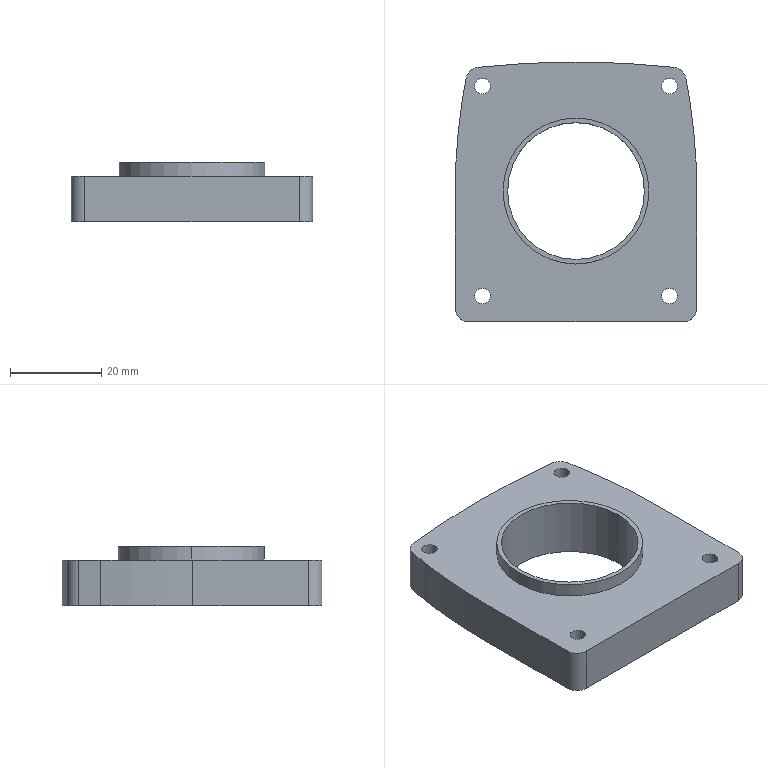Part | SolidWorks | features BaseBody 1 | 1 solid | 39 faces | box 53 x 57 x 13 mm | volume 21853 mm3 | cylinder 27 | plane 12 | commonest cylinder face diameters 6 x12 3.4 x8 30 x2 32 x2 267 x2 400 x1
STEP:
#1=CARTESIAN_POINT('',(15.,28.7,13.));
#2=VERTEX_POINT('',#1);
#3=CARTESIAN_POINT('',(-15.,28.7,13.));
#4=VERTEX_POINT('',#3);
#5=CARTESIAN_POINT('',(0.,28.7,13.));
#6=DIRECTION('',(0.,0.,-1.));
#7=DIRECTION('',(-1.,0.,0.));
#8=AXIS2_PLACEMENT_3D('',#5,#6,#7);
#9=CIRCLE('',#8,15.);
#10=EDGE_CURVE('',#2,#4,#9,.T.);
#11=ORIENTED_EDGE('',*,*,#10,.F.);
#12=CARTESIAN_POINT('',(15.,28.7,0.));
#13=VERTEX_POINT('',#12);
#14=CARTESIAN_POINT('',(15.,28.7,13.));
#15=DIRECTION('',(0.,0.,-1.));
#16=VECTOR('',#15,1000.);
#17=LINE('',#14,#16);
#18=EDGE_CURVE('',#2,#13,#17,.T.);
#19=ORIENTED_EDGE('',*,*,#18,.T.);
#20=CARTESIAN_POINT('',(-15.,28.7,0.));
#21=VERTEX_POINT('',#20);
#22=CARTESIAN_POINT('',(0.,28.7,0.));
#23=DIRECTION('',(0.,0.,-1.));
#24=DIRECTION('',(-1.,0.,0.));
#25=AXIS2_PLACEMENT_3D('',#22,#23,#24);
#26=CIRCLE('',#25,15.);
#27=EDGE_CURVE('',#13,#21,#26,.T.);
#28=ORIENTED_EDGE('',*,*,#27,.T.);
#29=CARTESIAN_POINT('',(-15.,28.7,13.));
#30=DIRECTION('',(0.,0.,-1.));
#31=VECTOR('',#30,1000.);
#32=LINE('',#29,#31);
#33=EDGE_CURVE('',#4,#21,#32,.T.);
#34=ORIENTED_EDGE('',*,*,#33,.F.);
#35=EDGE_LOOP('',(#11,#19,#28,#34));
#36=FACE_OUTER_BOUND('',#35,.T.);
#37=CARTESIAN_POINT('',(0.,28.7,13.));
#38=DIRECTION('',(0.,0.,-1.));
#39=DIRECTION('',(-1.,0.,0.));
#40=AXIS2_PLACEMENT_3D('',#37,#38,#39);
#41=CYLINDRICAL_SURFACE('',#40,15.);
#42=ADVANCED_FACE('',(#36),#41,.F.);
#43=CARTESIAN_POINT('',(-17.5,51.7,4.5));
#44=VERTEX_POINT('',#43);
#45=CARTESIAN_POINT('',(-23.5,51.7,4.5));
#46=VERTEX_POINT('',#45);
#47=CARTESIAN_POINT('',(-20.5,51.7,4.5));
#48=DIRECTION('',(0.,0.,-1.));
#49=DIRECTION('',(-1.,0.,0.));
#50=AXIS2_PLACEMENT_3D('',#47,#48,#49);
#51=CIRCLE('',#50,3.);
#52=EDGE_CURVE('',#44,#46,#51,.T.);
#53=ORIENTED_EDGE('',*,*,#52,.F.);
#54=CARTESIAN_POINT('',(-17.5,51.7,0.));
#55=VERTEX_POINT('',#54);
#56=CARTESIAN_POINT('',(-17.5,51.7,0.));
#57=DIRECTION('',(0.,0.,-1.));
#58=VECTOR('',#57,1000.);
#59=LINE('',#56,#58);
#60=EDGE_CURVE('',#44,#55,#59,.T.);
#61=ORIENTED_EDGE('',*,*,#60,.T.);
#62=CARTESIAN_POINT('',(-23.5,51.7,0.));
#63=VERTEX_POINT('',#62);
#64=CARTESIAN_POINT('',(-20.5,51.7,0.));
#65=DIRECTION('',(0.,0.,-1.));
#66=DIRECTION('',(-1.,0.,0.));
#67=AXIS2_PLACEMENT_3D('',#64,#65,#66);
#68=CIRCLE('',#67,3.);
#69=EDGE_CURVE('',#55,#63,#68,.T.);
#70=ORIENTED_EDGE('',*,*,#69,.T.);
#71=CARTESIAN_POINT('',(-23.5,51.7,0.));
#72=DIRECTION('',(0.,0.,-1.));
#73=VECTOR('',#72,1000.);
#74=LINE('',#71,#73);
#75=EDGE_CURVE('',#46,#63,#74,.T.);
#76=ORIENTED_EDGE('',*,*,#75,.F.);
#77=EDGE_LOOP('',(#53,#61,#70,#76));
#78=FACE_OUTER_BOUND('',#77,.T.);
#79=CARTESIAN_POINT('',(-20.5,51.7,0.));
#80=DIRECTION('',(0.,0.,-1.));
#81=DIRECTION('',(-1.,0.,0.));
#82=AXIS2_PLACEMENT_3D('',#79,#80,#81);
#83=CYLINDRICAL_SURFACE('',#82,3.);
#84=ADVANCED_FACE('',(#78),#83,.F.);
#85=CARTESIAN_POINT('',(-17.5,5.7,4.5));
#86=VERTEX_POINT('',#85);
#87=CARTESIAN_POINT('',(-23.5,5.7,4.5));
#88=VERTEX_POINT('',#87);
#89=CARTESIAN_POINT('',(-20.5,5.7,4.5));
#90=DIRECTION('',(0.,0.,-1.));
#91=DIRECTION('',(-1.,0.,0.));
#92=AXIS2_PLACEMENT_3D('',#89,#90,#91);
#93=CIRCLE('',#92,3.);
#94=EDGE_CURVE('',#86,#88,#93,.T.);
#95=ORIENTED_EDGE('',*,*,#94,.F.);
#96=CARTESIAN_POINT('',(-17.5,5.7,0.));
#97=VERTEX_POINT('',#96);
#98=CARTESIAN_POINT('',(-17.5,5.7,0.));
#99=DIRECTION('',(0.,0.,-1.));
#100=VECTOR('',#99,1000.);
#101=LINE('',#98,#100);
#102=EDGE_CURVE('',#86,#97,#101,.T.);
#103=ORIENTED_EDGE('',*,*,#102,.T.);
#104=CARTESIAN_POINT('',(-23.5,5.7,0.));
#105=VERTEX_POINT('',#104);
#106=CARTESIAN_POINT('',(-20.5,5.7,0.));
#107=DIRECTION('',(0.,0.,-1.));
#108=DIRECTION('',(-1.,0.,0.));
#109=AXIS2_PLACEMENT_3D('',#106,#107,#108);
#110=CIRCLE('',#109,3.);
#111=EDGE_CURVE('',#97,#105,#110,.T.);
#112=ORIENTED_EDGE('',*,*,#111,.T.);
#113=CARTESIAN_POINT('',(-23.5,5.7,0.));
#114=DIRECTION('',(0.,0.,-1.));
#115=VECTOR('',#114,1000.);
#116=LINE('',#113,#115);
#117=EDGE_CURVE('',#88,#105,#116,.T.);
#118=ORIENTED_EDGE('',*,*,#117,.F.);
#119=EDGE_LOOP('',(#95,#103,#112,#118));
#120=FACE_OUTER_BOUND('',#119,.T.);
#121=CARTESIAN_POINT('',(-20.5,5.7,0.));
#122=DIRECTION('',(0.,0.,-1.));
#123=DIRECTION('',(-1.,0.,0.));
#124=AXIS2_PLACEMENT_3D('',#121,#122,#123);
#125=CYLINDRICAL_SURFACE('',#124,3.);
#126=ADVANCED_FACE('',(#120),#125,.F.);
#127=CARTESIAN_POINT('',(23.5,5.7,4.5));
#128=VERTEX_POINT('',#127);
#129=CARTESIAN_POINT('',(17.5,5.7,4.5));
#130=VERTEX_POINT('',#129);
#131=CARTESIAN_POINT('',(20.5,5.7,4.5));
#132=DIRECTION('',(0.,0.,-1.));
#133=DIRECTION('',(-1.,0.,0.));
#134=AXIS2_PLACEMENT_3D('',#131,#132,#133);
#135=CIRCLE('',#134,3.);
#136=EDGE_CURVE('',#128,#130,#135,.T.);
#137=ORIENTED_EDGE('',*,*,#136,.F.);
#138=CARTESIAN_POINT('',(23.5,5.7,0.));
#139=VERTEX_POINT('',#138);
#140=CARTESIAN_POINT('',(23.5,5.7,0.));
#141=DIRECTION('',(0.,0.,-1.));
#142=VECTOR('',#141,1000.);
#143=LINE('',#140,#142);
#144=EDGE_CURVE('',#128,#139,#143,.T.);
#145=ORIENTED_EDGE('',*,*,#144,.T.);
#146=CARTESIAN_POINT('',(17.5,5.7,0.));
#147=VERTEX_POINT('',#146);
#148=CARTESIAN_POINT('',(20.5,5.7,0.));
#149=DIRECTION('',(0.,0.,-1.));
#150=DIRECTION('',(-1.,0.,0.));
#151=AXIS2_PLACEMENT_3D('',#148,#149,#150);
#152=CIRCLE('',#151,3.);
#153=EDGE_CURVE('',#139,#147,#152,.T.);
#154=ORIENTED_EDGE('',*,*,#153,.T.);
#155=CARTESIAN_POINT('',(17.5,5.7,0.));
#156=DIRECTION('',(0.,0.,-1.));
#157=VECTOR('',#156,1000.);
#158=LINE('',#155,#157);
#159=EDGE_CURVE('',#130,#147,#158,.T.);
#160=ORIENTED_EDGE('',*,*,#159,.F.);
#161=EDGE_LOOP('',(#137,#145,#154,#160));
#162=FACE_OUTER_BOUND('',#161,.T.);
#163=CARTESIAN_POINT('',(20.5,5.7,0.));
#164=DIRECTION('',(0.,0.,-1.));
#165=DIRECTION('',(-1.,0.,0.));
#166=AXIS2_PLACEMENT_3D('',#163,#164,#165);
#167=CYLINDRICAL_SURFACE('',#166,3.);
#168=ADVANCED_FACE('',(#162),#167,.F.);
#169=CARTESIAN_POINT('',(23.5,51.7,4.5));
#170=VERTEX_POINT('',#169);
#171=CARTESIAN_POINT('',(17.5,51.7,4.5));
#172=VERTEX_POINT('',#171);
#173=CARTESIAN_POINT('',(20.5,51.7,4.5));
#174=DIRECTION('',(0.,0.,-1.));
#175=DIRECTION('',(-1.,0.,0.));
#176=AXIS2_PLACEMENT_3D('',#173,#174,#175);
#177=CIRCLE('',#176,3.);
#178=EDGE_CURVE('',#170,#172,#177,.T.);
#179=ORIENTED_EDGE('',*,*,#178,.F.);
#180=CARTESIAN_POINT('',(23.5,51.7,0.));
#181=VERTEX_POINT('',#180);
#182=CARTESIAN_POINT('',(23.5,51.7,0.));
#183=DIRECTION('',(0.,0.,-1.));
#184=VECTOR('',#183,1000.);
#185=LINE('',#182,#184);
#186=EDGE_CURVE('',#170,#181,#185,.T.);
#187=ORIENTED_EDGE('',*,*,#186,.T.);
#188=CARTESIAN_POINT('',(17.5,51.7,0.));
#189=VERTEX_POINT('',#188);
#190=CARTESIAN_POINT('',(20.5,51.7,0.));
#191=DIRECTION('',(0.,0.,-1.));
#192=DIRECTION('',(-1.,0.,0.));
#193=AXIS2_PLACEMENT_3D('',#190,#191,#192);
#194=CIRCLE('',#193,3.);
#195=EDGE_CURVE('',#181,#189,#194,.T.);
#196=ORIENTED_EDGE('',*,*,#195,.T.);
#197=CARTESIAN_POINT('',(17.5,51.7,0.));
#198=DIRECTION('',(0.,0.,-1.));
#199=VECTOR('',#198,1000.);
#200=LINE('',#197,#199);
#201=EDGE_CURVE('',#172,#189,#200,.T.);
#202=ORIENTED_EDGE('',*,*,#201,.F.);
#203=EDGE_LOOP('',(#179,#187,#196,#202));
#204=FACE_OUTER_BOUND('',#203,.T.);
#205=CARTESIAN_POINT('',(20.5,51.7,0.));
#206=DIRECTION('',(0.,0.,-1.));
#207=DIRECTION('',(-1.,0.,0.));
#208=AXIS2_PLACEMENT_3D('',#205,#206,#207);
#209=CYLINDRICAL_SURFACE('',#208,3.);
#210=ADVANCED_FACE('',(#204),#209,.F.);
#211=CARTESIAN_POINT('',(16.,28.7,13.));
#212=VERTEX_POINT('',#211);
#213=CARTESIAN_POINT('',(-16.,28.7,13.));
#214=VERTEX_POINT('',#213);
#215=CARTESIAN_POINT('',(0.,28.7,13.));
#216=DIRECTION('',(0.,0.,1.));
#217=DIRECTION('',(-1.,0.,0.));
#218=AXIS2_PLACEMENT_3D('',#215,#216,#217);
#219=CIRCLE('',#218,16.);
#220=EDGE_CURVE('',#212,#214,#219,.T.);
#221=ORIENTED_EDGE('',*,*,#220,.F.);
#222=CARTESIAN_POINT('',(16.,28.7,10.));
#223=VERTEX_POINT('',#222);
#224=CARTESIAN_POINT('',(16.,28.7,13.));
#225=DIRECTION('',(0.,0.,-1.));
#226=VECTOR('',#225,1000.);
#227=LINE('',#224,#226);
#228=EDGE_CURVE('',#212,#223,#227,.T.);
#229=ORIENTED_EDGE('',*,*,#228,.T.);
#230=CARTESIAN_POINT('',(-16.,28.7,10.));
#231=VERTEX_POINT('',#230);
#232=CARTESIAN_POINT('',(0.,28.7,10.));
#233=DIRECTION('',(0.,0.,-1.));
#234=DIRECTION('',(-1.,0.,0.));
#235=AXIS2_PLACEMENT_3D('',#232,#233,#234);
#236=CIRCLE('',#235,16.);
#237=EDGE_CURVE('',#231,#223,#236,.T.);
#238=ORIENTED_EDGE('',*,*,#237,.F.);
#239=CARTESIAN_POINT('',(-16.,28.7,13.));
#240=DIRECTION('',(0.,0.,-1.));
#241=VECTOR('',#240,1000.);
#242=LINE('',#239,#241);
#243=EDGE_CURVE('',#214,#231,#242,.T.);
#244=ORIENTED_EDGE('',*,*,#243,.F.);
#245=EDGE_LOOP('',(#221,#229,#238,#244));
#246=FACE_OUTER_BOUND('',#245,.T.);
#247=CARTESIAN_POINT('',(0.,28.7,13.));
#248=DIRECTION('',(0.,0.,-1.));
#249=DIRECTION('',(-1.,0.,0.));
#250=AXIS2_PLACEMENT_3D('',#247,#248,#249);
#251=CYLINDRICAL_SURFACE('',#250,16.);
#252=ADVANCED_FACE('',(#246),#251,.T.);
#253=CARTESIAN_POINT('',(-18.8,51.7,10.));
#254=VERTEX_POINT('',#253);
#255=CARTESIAN_POINT('',(-22.2,51.7,10.));
#256=VERTEX_POINT('',#255);
#257=CARTESIAN_POINT('',(-20.5,51.7,10.));
#258=DIRECTION('',(0.,0.,-1.));
#259=DIRECTION('',(-1.,0.,0.));
#260=AXIS2_PLACEMENT_3D('',#257,#258,#259);
#261=CIRCLE('',#260,1.7);
#262=EDGE_CURVE('',#254,#256,#261,.T.);
#263=ORIENTED_EDGE('',*,*,#262,.F.);
#264=CARTESIAN_POINT('',(-18.8,51.7,4.5));
#265=VERTEX_POINT('',#264);
#266=CARTESIAN_POINT('',(-18.8,51.7,0.));
#267=DIRECTION('',(0.,0.,-1.));
#268=VECTOR('',#267,1000.);
#269=LINE('',#266,#268);
#270=EDGE_CURVE('',#254,#265,#269,.T.);
#271=ORIENTED_EDGE('',*,*,#270,.T.);
#272=CARTESIAN_POINT('',(-22.2,51.7,4.5));
#273=VERTEX_POINT('',#272);
#274=CARTESIAN_POINT('',(-20.5,51.7,4.5));
#275=DIRECTION('',(0.,0.,-1.));
#276=DIRECTION('',(-1.,0.,0.));
#277=AXIS2_PLACEMENT_3D('',#274,#275,#276);
#278=CIRCLE('',#277,1.7);
#279=EDGE_CURVE('',#265,#273,#278,.T.);
#280=ORIENTED_EDGE('',*,*,#279,.T.);
#281=CARTESIAN_POINT('',(-22.2,51.7,0.));
#282=DIRECTION('',(0.,0.,-1.));
#283=VECTOR('',#282,1000.);
#284=LINE('',#281,#283);
#285=EDGE_CURVE('',#256,#273,#284,.T.);
#286=ORIENTED_EDGE('',*,*,#285,.F.);
#287=EDGE_LOOP('',(#263,#271,#280,#286));
#288=FACE_OUTER_BOUND('',#287,.T.);
#289=CARTESIAN_POINT('',(-20.5,51.7,0.));
#290=DIRECTION('',(0.,0.,-1.));
#291=DIRECTION('',(-1.,0.,0.));
#292=AXIS2_PLACEMENT_3D('',#289,#290,#291);
#293=CYLINDRICAL_SURFACE('',#292,1.7);
#294=ADVANCED_FACE('',(#288),#293,.F.);
#295=CARTESIAN_POINT('',(-18.8,5.7,10.));
#296=VERTEX_POINT('',#295);
#297=CARTESIAN_POINT('',(-22.2,5.7,10.));
#298=VERTEX_POINT('',#297);
#299=CARTESIAN_POINT('',(-20.5,5.7,10.));
#300=DIRECTION('',(0.,0.,-1.));
#301=DIRECTION('',(-1.,0.,0.));
#302=AXIS2_PLACEMENT_3D('',#299,#300,#301);
#303=CIRCLE('',#302,1.7);
#304=EDGE_CURVE('',#296,#298,#303,.T.);
#305=ORIENTED_EDGE('',*,*,#304,.F.);
#306=CARTESIAN_POINT('',(-18.8,5.7,4.5));
#307=VERTEX_POINT('',#306);
#308=CARTESIAN_POINT('',(-18.8,5.7,0.));
#309=DIRECTION('',(0.,0.,-1.));
#310=VECTOR('',#309,1000.);
#311=LINE('',#308,#310);
#312=EDGE_CURVE('',#296,#307,#311,.T.);
#313=ORIENTED_EDGE('',*,*,#312,.T.);
#314=CARTESIAN_POINT('',(-22.2,5.7,4.5));
#315=VERTEX_POINT('',#314);
#316=CARTESIAN_POINT('',(-20.5,5.7,4.5));
#317=DIRECTION('',(0.,0.,-1.));
#318=DIRECTION('',(-1.,0.,0.));
#319=AXIS2_PLACEMENT_3D('',#316,#317,#318);
#320=CIRCLE('',#319,1.7);
#321=EDGE_CURVE('',#307,#315,#320,.T.);
#322=ORIENTED_EDGE('',*,*,#321,.T.);
#323=CARTESIAN_POINT('',(-22.2,5.7,0.));
#324=DIRECTION('',(0.,0.,-1.));
#325=VECTOR('',#324,1000.);
#326=LINE('',#323,#325);
#327=EDGE_CURVE('',#298,#315,#326,.T.);
#328=ORIENTED_EDGE('',*,*,#327,.F.);
#329=EDGE_LOOP('',(#305,#313,#322,#328));
#330=FACE_OUTER_BOUND('',#329,.T.);
#331=CARTESIAN_POINT('',(-20.5,5.7,0.));
#332=DIRECTION('',(0.,0.,-1.));
#333=DIRECTION('',(-1.,0.,0.));
#334=AXIS2_PLACEMENT_3D('',#331,#332,#333);
#335=CYLINDRICAL_SURFACE('',#334,1.7);
#336=ADVANCED_FACE('',(#330),#335,.F.);
#337=CARTESIAN_POINT('',(22.2,5.7,10.));
#338=VERTEX_POINT('',#337);
#339=CARTESIAN_POINT('',(18.8,5.7,10.));
#340=VERTEX_POINT('',#339);
#341=CARTESIAN_POINT('',(20.5,5.7,10.));
#342=DIRECTION('',(0.,0.,-1.));
#343=DIRECTION('',(-1.,0.,0.));
#344=AXIS2_PLACEMENT_3D('',#341,#342,#343);
#345=CIRCLE('',#344,1.7);
#346=EDGE_CURVE('',#338,#340,#345,.T.);
#347=ORIENTED_EDGE('',*,*,#346,.F.);
#348=CARTESIAN_POINT('',(22.2,5.7,4.5));
#349=VERTEX_POINT('',#348);
#350=CARTESIAN_POINT('',(22.2,5.7,0.));
#351=DIRECTION('',(0.,0.,-1.));
#352=VECTOR('',#351,1000.);
#353=LINE('',#350,#352);
#354=EDGE_CURVE('',#338,#349,#353,.T.);
#355=ORIENTED_EDGE('',*,*,#354,.T.);
#356=CARTESIAN_POINT('',(18.8,5.7,4.5));
#357=VERTEX_POINT('',#356);
#358=CARTESIAN_POINT('',(20.5,5.7,4.5));
#359=DIRECTION('',(0.,0.,-1.));
#360=DIRECTION('',(-1.,0.,0.));
#361=AXIS2_PLACEMENT_3D('',#358,#359,#360);
#362=CIRCLE('',#361,1.7);
#363=EDGE_CURVE('',#349,#357,#362,.T.);
#364=ORIENTED_EDGE('',*,*,#363,.T.);
#365=CARTESIAN_POINT('',(18.8,5.7,0.));
#366=DIRECTION('',(0.,0.,-1.));
#367=VECTOR('',#366,1000.);
#368=LINE('',#365,#367);
#369=EDGE_CURVE('',#340,#357,#368,.T.);
#370=ORIENTED_EDGE('',*,*,#369,.F.);
#371=EDGE_LOOP('',(#347,#355,#364,#370));
#372=FACE_OUTER_BOUND('',#371,.T.);
#373=CARTESIAN_POINT('',(20.5,5.7,0.));
#374=DIRECTION('',(0.,0.,-1.));
#375=DIRECTION('',(-1.,0.,0.));
#376=AXIS2_PLACEMENT_3D('',#373,#374,#375);
#377=CYLINDRICAL_SURFACE('',#376,1.7);
#378=ADVANCED_FACE('',(#372),#377,.F.);
#379=CARTESIAN_POINT('',(22.2,51.7,10.));
#380=VERTEX_POINT('',#379);
#381=CARTESIAN_POINT('',(18.8,51.7,10.));
#382=VERTEX_POINT('',#381);
#383=CARTESIAN_POINT('',(20.5,51.7,10.));
#384=DIRECTION('',(0.,0.,-1.));
#385=DIRECTION('',(-1.,0.,0.));
#386=AXIS2_PLACEMENT_3D('',#383,#384,#385);
#387=CIRCLE('',#386,1.7);
#388=EDGE_CURVE('',#380,#382,#387,.T.);
#389=ORIENTED_EDGE('',*,*,#388,.F.);
#390=CARTESIAN_POINT('',(22.2,51.7,4.5));
#391=VERTEX_POINT('',#390);
#392=CARTESIAN_POINT('',(22.2,51.7,0.));
#393=DIRECTION('',(0.,0.,-1.));
#394=VECTOR('',#393,1000.);
#395=LINE('',#392,#394);
#396=EDGE_CURVE('',#380,#391,#395,.T.);
#397=ORIENTED_EDGE('',*,*,#396,.T.);
#398=CARTESIAN_POINT('',(18.8,51.7,4.5));
#399=VERTEX_POINT('',#398);
#400=CARTESIAN_POINT('',(20.5,51.7,4.5));
#401=DIRECTION('',(0.,0.,-1.));
#402=DIRECTION('',(-1.,0.,0.));
#403=AXIS2_PLACEMENT_3D('',#400,#401,#402);
#404=CIRCLE('',#403,1.7);
#405=EDGE_CURVE('',#391,#399,#404,.T.);
#406=ORIENTED_EDGE('',*,*,#405,.T.);
#407=CARTESIAN_POINT('',(18.8,51.7,0.));
#408=DIRECTION('',(0.,0.,-1.));
#409=VECTOR('',#408,1000.);
#410=LINE('',#407,#409);
#411=EDGE_CURVE('',#382,#399,#410,.T.);
#412=ORIENTED_EDGE('',*,*,#411,.F.);
#413=EDGE_LOOP('',(#389,#397,#406,#412));
#414=FACE_OUTER_BOUND('',#413,.T.);
#415=CARTESIAN_POINT('',(20.5,51.7,0.));
#416=DIRECTION('',(0.,0.,-1.));
#417=DIRECTION('',(-1.,0.,0.));
#418=AXIS2_PLACEMENT_3D('',#415,#416,#417);
#419=CYLINDRICAL_SURFACE('',#418,1.7);
#420=ADVANCED_FACE('',(#414),#419,.F.);
#421=CARTESIAN_POINT('',(-23.5,0.,0.));
#422=VERTEX_POINT('',#421);
#423=CARTESIAN_POINT('',(23.5,0.,0.));
#424=VERTEX_POINT('',#423);
#425=CARTESIAN_POINT('',(23.5,0.,0.));
#426=DIRECTION('',(1.,0.,0.));
#427=VECTOR('',#426,1000.);
#428=LINE('',#425,#427);
#429=EDGE_CURVE('',#422,#424,#428,.T.);
#430=ORIENTED_EDGE('',*,*,#429,.F.);
#431=CARTESIAN_POINT('',(-26.5,3.,0.));
#432=VERTEX_POINT('',#431);
#433=CARTESIAN_POINT('',(-23.5,3.,0.));
#434=DIRECTION('',(0.,0.,1.));
#435=DIRECTION('',(-1.,0.,0.));
#436=AXIS2_PLACEMENT_3D('',#433,#434,#435);
#437=CIRCLE('',#436,3.);
#438=EDGE_CURVE('',#432,#422,#437,.T.);
#439=ORIENTED_EDGE('',*,*,#438,.F.);
#440=CARTESIAN_POINT('',(-26.5,28.3,0.));
#441=VERTEX_POINT('',#440);
#442=CARTESIAN_POINT('',(-26.5,3.,0.));
#443=DIRECTION('',(0.,-1.,0.));
#444=VECTOR('',#443,1000.);
#445=LINE('',#442,#444);
#446=EDGE_CURVE('',#441,#432,#445,.T.);
#447=ORIENTED_EDGE('',*,*,#446,.F.);
#448=CARTESIAN_POINT('',(-24.963,48.5,0.));
#449=VERTEX_POINT('',#448);
#450=CARTESIAN_POINT('',(107.,28.3,0.));
#451=DIRECTION('',(0.,0.,1.));
#452=DIRECTION('',(-1.,0.,0.));
#453=AXIS2_PLACEMENT_3D('',#450,#451,#452);
#454=CIRCLE('',#453,133.5);
#455=EDGE_CURVE('',#449,#441,#454,.T.);
#456=ORIENTED_EDGE('',*,*,#455,.F.);
#457=CARTESIAN_POINT('',(-24.102,53.383,0.));
#458=VERTEX_POINT('',#457);
#459=CARTESIAN_POINT('',(-24.102,53.383,0.));
#460=DIRECTION('',(-0.1736,-0.9848,0.));
#461=VECTOR('',#460,1000.);
#462=LINE('',#459,#461);
#463=EDGE_CURVE('',#458,#449,#462,.T.);
#464=ORIENTED_EDGE('',*,*,#463,.F.);
#465=CARTESIAN_POINT('',(-21.47,55.844,0.));
#466=VERTEX_POINT('',#465);
#467=CARTESIAN_POINT('',(-21.148,52.862,0.));
#468=DIRECTION('',(0.,0.,1.));
#469=DIRECTION('',(-1.,0.,0.));
#470=AXIS2_PLACEMENT_3D('',#467,#468,#469);
#471=CIRCLE('',#470,3.);
#472=EDGE_CURVE('',#466,#458,#471,.T.);
#473=ORIENTED_EDGE('',*,*,#472,.F.);
#474=CARTESIAN_POINT('',(21.47,55.844,0.));
#475=VERTEX_POINT('',#474);
#476=CARTESIAN_POINT('',(0.,-143.,0.));
#477=DIRECTION('',(0.,0.,1.));
#478=DIRECTION('',(-1.,0.,0.));
#479=AXIS2_PLACEMENT_3D('',#476,#477,#478);
#480=CIRCLE('',#479,200.);
#481=EDGE_CURVE('',#475,#466,#480,.T.);
#482=ORIENTED_EDGE('',*,*,#481,.F.);
#483=CARTESIAN_POINT('',(24.102,53.383,0.));
#484=VERTEX_POINT('',#483);
#485=CARTESIAN_POINT('',(21.148,52.862,0.));
#486=DIRECTION('',(0.,0.,1.));
#487=DIRECTION('',(-1.,0.,0.));
#488=AXIS2_PLACEMENT_3D('',#485,#486,#487);
#489=CIRCLE('',#488,3.);
#490=EDGE_CURVE('',#484,#475,#489,.T.);
#491=ORIENTED_EDGE('',*,*,#490,.F.);
#492=CARTESIAN_POINT('',(24.963,48.5,0.));
#493=VERTEX_POINT('',#492);
#494=CARTESIAN_POINT('',(24.963,48.5,0.));
#495=DIRECTION('',(-0.1736,0.9848,0.));
#496=VECTOR('',#495,1000.);
#497=LINE('',#494,#496);
#498=EDGE_CURVE('',#493,#484,#497,.T.);
#499=ORIENTED_EDGE('',*,*,#498,.F.);
#500=CARTESIAN_POINT('',(26.5,28.3,0.));
#501=VERTEX_POINT('',#500);
#502=CARTESIAN_POINT('',(-107.,28.3,0.));
#503=DIRECTION('',(0.,0.,1.));
#504=DIRECTION('',(-1.,0.,0.));
#505=AXIS2_PLACEMENT_3D('',#502,#503,#504);
#506=CIRCLE('',#505,133.5);
#507=EDGE_CURVE('',#501,#493,#506,.T.);
#508=ORIENTED_EDGE('',*,*,#507,.F.);
#509=CARTESIAN_POINT('',(26.5,3.,0.));
#510=VERTEX_POINT('',#509);
#511=CARTESIAN_POINT('',(26.5,3.,0.));
#512=DIRECTION('',(0.,1.,0.));
#513=VECTOR('',#512,1000.);
#514=LINE('',#511,#513);
#515=EDGE_CURVE('',#510,#501,#514,.T.);
#516=ORIENTED_EDGE('',*,*,#515,.F.);
#517=CARTESIAN_POINT('',(23.5,3.,0.));
#518=DIRECTION('',(0.,0.,1.));
#519=DIRECTION('',(-1.,0.,0.));
#520=AXIS2_PLACEMENT_3D('',#517,#518,#519);
#521=CIRCLE('',#520,3.);
#522=EDGE_CURVE('',#424,#510,#521,.T.);
#523=ORIENTED_EDGE('',*,*,#522,.F.);
#524=EDGE_LOOP('',(#430,#439,#447,#456,#464,#473,#482,#491,#499,#508,#516,#523));
#525=FACE_OUTER_BOUND('',#524,.T.);
#526=CARTESIAN_POINT('',(0.,28.7,0.));
#527=DIRECTION('',(0.,0.,-1.));
#528=DIRECTION('',(-1.,0.,0.));
#529=AXIS2_PLACEMENT_3D('',#526,#527,#528);
#530=CIRCLE('',#529,15.);
#531=EDGE_CURVE('',#21,#13,#530,.T.);
#532=ORIENTED_EDGE('',*,*,#531,.F.);
#533=ORIENTED_EDGE('',*,*,#27,.F.);
#534=EDGE_LOOP('',(#532,#533));
#535=FACE_BOUND('',#534,.T.);
#536=CARTESIAN_POINT('',(-20.5,51.7,0.));
#537=DIRECTION('',(0.,0.,-1.));
#538=DIRECTION('',(-1.,0.,0.));
#539=AXIS2_PLACEMENT_3D('',#536,#537,#538);
#540=CIRCLE('',#539,3.);
#541=EDGE_CURVE('',#63,#55,#540,.T.);
#542=ORIENTED_EDGE('',*,*,#541,.F.);
#543=ORIENTED_EDGE('',*,*,#69,.F.);
#544=EDGE_LOOP('',(#542,#543));
#545=FACE_BOUND('',#544,.T.);
#546=CARTESIAN_POINT('',(-20.5,5.7,0.));
#547=DIRECTION('',(0.,0.,-1.));
#548=DIRECTION('',(-1.,0.,0.));
#549=AXIS2_PLACEMENT_3D('',#546,#547,#548);
#550=CIRCLE('',#549,3.);
#551=EDGE_CURVE('',#105,#97,#550,.T.);
#552=ORIENTED_EDGE('',*,*,#551,.F.);
#553=ORIENTED_EDGE('',*,*,#111,.F.);
#554=EDGE_LOOP('',(#552,#553));
#555=FACE_BOUND('',#554,.T.);
#556=CARTESIAN_POINT('',(20.5,5.7,0.));
#557=DIRECTION('',(0.,0.,-1.));
#558=DIRECTION('',(-1.,0.,0.));
#559=AXIS2_PLACEMENT_3D('',#556,#557,#558);
#560=CIRCLE('',#559,3.);
#561=EDGE_CURVE('',#147,#139,#560,.T.);
#562=ORIENTED_EDGE('',*,*,#561,.F.);
#563=ORIENTED_EDGE('',*,*,#153,.F.);
#564=EDGE_LOOP('',(#562,#563));
#565=FACE_BOUND('',#564,.T.);
#566=CARTESIAN_POINT('',(20.5,51.7,0.));
#567=DIRECTION('',(0.,0.,-1.));
#568=DIRECTION('',(-1.,0.,0.));
#569=AXIS2_PLACEMENT_3D('',#566,#567,#568);
#570=CIRCLE('',#569,3.);
#571=EDGE_CURVE('',#189,#181,#570,.T.);
#572=ORIENTED_EDGE('',*,*,#571,.F.);
#573=ORIENTED_EDGE('',*,*,#195,.F.);
#574=EDGE_LOOP('',(#572,#573));
#575=FACE_BOUND('',#574,.T.);
#576=CARTESIAN_POINT('',(23.5,3.,0.));
#577=DIRECTION('',(0.,0.,1.));
#578=DIRECTION('',(1.,0.,0.));
#579=AXIS2_PLACEMENT_3D('',#576,#577,#578);
#580=PLANE('',#579);
#581=ADVANCED_FACE('',(#525,#535,#545,#555,#565,#575),#580,.F.);
#582=CARTESIAN_POINT('',(26.5,3.,10.));
#583=VERTEX_POINT('',#582);
#584=CARTESIAN_POINT('',(23.5,0.,10.));
#585=VERTEX_POINT('',#584);
#586=CARTESIAN_POINT('',(23.5,3.,10.));
#587=DIRECTION('',(0.,0.,-1.));
#588=DIRECTION('',(-1.,0.,0.));
#589=AXIS2_PLACEMENT_3D('',#586,#587,#588);
#590=CIRCLE('',#589,3.);
#591=EDGE_CURVE('',#583,#585,#590,.T.);
#592=ORIENTED_EDGE('',*,*,#591,.T.);
#593=CARTESIAN_POINT('',(23.5,0.,10.));
#594=DIRECTION('',(0.,0.,-1.));
#595=VECTOR('',#594,1000.);
#596=LINE('',#593,#595);
#597=EDGE_CURVE('',#585,#424,#596,.T.);
#598=ORIENTED_EDGE('',*,*,#597,.T.);
#599=ORIENTED_EDGE('',*,*,#522,.T.);
#600=CARTESIAN_POINT('',(26.5,3.,10.));
#601=DIRECTION('',(0.,0.,1.));
#602=VECTOR('',#601,1000.);
#603=LINE('',#600,#602);
#604=EDGE_CURVE('',#510,#583,#603,.T.);
#605=ORIENTED_EDGE('',*,*,#604,.T.);
#606=EDGE_LOOP('',(#592,#598,#599,#605));
#607=FACE_OUTER_BOUND('',#606,.T.);
#608=CARTESIAN_POINT('',(23.5,3.,10.));
#609=DIRECTION('',(0.,0.,-1.));
#610=DIRECTION('',(-1.,0.,0.));
#611=AXIS2_PLACEMENT_3D('',#608,#609,#610);
#612=CYLINDRICAL_SURFACE('',#611,3.);
#613=ADVANCED_FACE('',(#607),#612,.T.);
#614=ORIENTED_EDGE('',*,*,#597,.F.);
#615=CARTESIAN_POINT('',(-23.5,0.,10.));
#616=VERTEX_POINT('',#615);
#617=CARTESIAN_POINT('',(23.5,0.,10.));
#618=DIRECTION('',(1.,0.,0.));
#619=VECTOR('',#618,1000.);
#620=LINE('',#617,#619);
#621=EDGE_CURVE('',#616,#585,#620,.T.);
#622=ORIENTED_EDGE('',*,*,#621,.F.);
#623=CARTESIAN_POINT('',(-23.5,0.,10.));
#624=DIRECTION('',(0.,0.,1.));
#625=VECTOR('',#624,1000.);
#626=LINE('',#623,#625);
#627=EDGE_CURVE('',#422,#616,#626,.T.);
#628=ORIENTED_EDGE('',*,*,#627,.F.);
#629=ORIENTED_EDGE('',*,*,#429,.T.);
#630=EDGE_LOOP('',(#614,#622,#628,#629));
#631=FACE_OUTER_BOUND('',#630,.T.);
#632=CARTESIAN_POINT('',(23.5,0.,10.));
#633=DIRECTION('',(0.,1.,0.));
#634=DIRECTION('',(0.,0.,1.));
#635=AXIS2_PLACEMENT_3D('',#632,#633,#634);
#636=PLANE('',#635);
#637=ADVANCED_FACE('',(#631),#636,.F.);
#638=CARTESIAN_POINT('',(-26.5,3.,10.));
#639=VERTEX_POINT('',#638);
#640=CARTESIAN_POINT('',(-23.5,3.,10.));
#641=DIRECTION('',(0.,0.,-1.));
#642=DIRECTION('',(-1.,0.,0.));
#643=AXIS2_PLACEMENT_3D('',#640,#641,#642);
#644=CIRCLE('',#643,3.);
#645=EDGE_CURVE('',#616,#639,#644,.T.);
#646=ORIENTED_EDGE('',*,*,#645,.T.);
#647=CARTESIAN_POINT('',(-26.5,3.,10.));
#648=DIRECTION('',(0.,0.,-1.));
#649=VECTOR('',#648,1000.);
#650=LINE('',#647,#649);
#651=EDGE_CURVE('',#639,#432,#650,.T.);
#652=ORIENTED_EDGE('',*,*,#651,.T.);
#653=ORIENTED_EDGE('',*,*,#438,.T.);
#654=ORIENTED_EDGE('',*,*,#627,.T.);
#655=EDGE_LOOP('',(#646,#652,#653,#654));
#656=FACE_OUTER_BOUND('',#655,.T.);
#657=CARTESIAN_POINT('',(-23.5,3.,10.));
#658=DIRECTION('',(0.,0.,-1.));
#659=DIRECTION('',(-1.,0.,0.));
#660=AXIS2_PLACEMENT_3D('',#657,#658,#659);
#661=CYLINDRICAL_SURFACE('',#660,3.);
#662=ADVANCED_FACE('',(#656),#661,.T.);
#663=ORIENTED_EDGE('',*,*,#651,.F.);
#664=CARTESIAN_POINT('',(-26.5,28.3,10.));
#665=VERTEX_POINT('',#664);
#666=CARTESIAN_POINT('',(-26.5,3.,10.));
#667=DIRECTION('',(0.,-1.,0.));
#668=VECTOR('',#667,1000.);
#669=LINE('',#666,#668);
#670=EDGE_CURVE('',#665,#639,#669,.T.);
#671=ORIENTED_EDGE('',*,*,#670,.F.);
#672=CARTESIAN_POINT('',(-26.5,28.3,10.));
#673=DIRECTION('',(0.,0.,1.));
#674=VECTOR('',#673,1000.);
#675=LINE('',#672,#674);
#676=EDGE_CURVE('',#441,#665,#675,.T.);
#677=ORIENTED_EDGE('',*,*,#676,.F.);
#678=ORIENTED_EDGE('',*,*,#446,.T.);
#679=EDGE_LOOP('',(#663,#671,#677,#678));
#680=FACE_OUTER_BOUND('',#679,.T.);
#681=CARTESIAN_POINT('',(-26.5,3.,10.));
#682=DIRECTION('',(1.,0.,0.));
#683=DIRECTION('',(0.,0.,-1.));
#684=AXIS2_PLACEMENT_3D('',#681,#682,#683);
#685=PLANE('',#684);
#686=ADVANCED_FACE('',(#680),#685,.F.);
#687=CARTESIAN_POINT('',(-24.963,48.5,10.));
#688=VERTEX_POINT('',#687);
#689=CARTESIAN_POINT('',(107.,28.3,10.));
#690=DIRECTION('',(0.,0.,-1.));
#691=DIRECTION('',(-1.,0.,0.));
#692=AXIS2_PLACEMENT_3D('',#689,#690,#691);
#693=CIRCLE('',#692,133.5);
#694=EDGE_CURVE('',#665,#688,#693,.T.);
#695=ORIENTED_EDGE('',*,*,#694,.T.);
#696=CARTESIAN_POINT('',(-24.963,48.5,10.));
#697=DIRECTION('',(0.,0.,-1.));
#698=VECTOR('',#697,1000.);
#699=LINE('',#696,#698);
#700=EDGE_CURVE('',#688,#449,#699,.T.);
#701=ORIENTED_EDGE('',*,*,#700,.T.);
#702=ORIENTED_EDGE('',*,*,#455,.T.);
#703=ORIENTED_EDGE('',*,*,#676,.T.);
#704=EDGE_LOOP('',(#695,#701,#702,#703));
#705=FACE_OUTER_BOUND('',#704,.T.);
#706=CARTESIAN_POINT('',(107.,28.3,10.));
#707=DIRECTION('',(0.,0.,-1.));
#708=DIRECTION('',(-1.,0.,0.));
#709=AXIS2_PLACEMENT_3D('',#706,#707,#708);
#710=CYLINDRICAL_SURFACE('',#709,133.5);
#711=ADVANCED_FACE('',(#705),#710,.T.);
#712=ORIENTED_EDGE('',*,*,#700,.F.);
#713=CARTESIAN_POINT('',(-24.102,53.383,10.));
#714=VERTEX_POINT('',#713);
#715=CARTESIAN_POINT('',(-24.963,48.5,10.));
#716=DIRECTION('',(-0.1736,-0.9848,0.));
#717=VECTOR('',#716,1000.);
#718=LINE('',#715,#717);
#719=EDGE_CURVE('',#714,#688,#718,.T.);
#720=ORIENTED_EDGE('',*,*,#719,.F.);
#721=CARTESIAN_POINT('',(-24.102,53.383,10.));
#722=DIRECTION('',(0.,0.,1.));
#723=VECTOR('',#722,1000.);
#724=LINE('',#721,#723);
#725=EDGE_CURVE('',#458,#714,#724,.T.);
#726=ORIENTED_EDGE('',*,*,#725,.F.);
#727=ORIENTED_EDGE('',*,*,#463,.T.);
#728=EDGE_LOOP('',(#712,#720,#726,#727));
#729=FACE_OUTER_BOUND('',#728,.T.);
#730=CARTESIAN_POINT('',(-24.963,48.5,10.));
#731=DIRECTION('',(0.9848,-0.1736,0.));
#732=DIRECTION('',(0.1736,0.9848,0.));
#733=AXIS2_PLACEMENT_3D('',#730,#731,#732);
#734=PLANE('',#733);
#735=ADVANCED_FACE('',(#729),#734,.F.);
#736=CARTESIAN_POINT('',(-21.47,55.844,10.));
#737=VERTEX_POINT('',#736);
#738=CARTESIAN_POINT('',(-21.148,52.862,10.));
#739=DIRECTION('',(0.,0.,-1.));
#740=DIRECTION('',(-1.,0.,0.));
#741=AXIS2_PLACEMENT_3D('',#738,#739,#740);
#742=CIRCLE('',#741,3.);
#743=EDGE_CURVE('',#714,#737,#742,.T.);
#744=ORIENTED_EDGE('',*,*,#743,.T.);
#745=CARTESIAN_POINT('',(-21.47,55.844,10.));
#746=DIRECTION('',(0.,0.,-1.));
#747=VECTOR('',#746,1000.);
#748=LINE('',#745,#747);
#749=EDGE_CURVE('',#737,#466,#748,.T.);
#750=ORIENTED_EDGE('',*,*,#749,.T.);
#751=ORIENTED_EDGE('',*,*,#472,.T.);
#752=ORIENTED_EDGE('',*,*,#725,.T.);
#753=EDGE_LOOP('',(#744,#750,#751,#752));
#754=FACE_OUTER_BOUND('',#753,.T.);
#755=CARTESIAN_POINT('',(-21.148,52.862,10.));
#756=DIRECTION('',(0.,0.,-1.));
#757=DIRECTION('',(-1.,0.,0.));
#758=AXIS2_PLACEMENT_3D('',#755,#756,#757);
#759=CYLINDRICAL_SURFACE('',#758,3.);
#760=ADVANCED_FACE('',(#754),#759,.T.);
#761=CARTESIAN_POINT('',(21.47,55.844,10.));
#762=VERTEX_POINT('',#761);
#763=CARTESIAN_POINT('',(0.,-143.,10.));
#764=DIRECTION('',(0.,0.,-1.));
#765=DIRECTION('',(-1.,0.,0.));
#766=AXIS2_PLACEMENT_3D('',#763,#764,#765);
#767=CIRCLE('',#766,200.);
#768=EDGE_CURVE('',#737,#762,#767,.T.);
#769=ORIENTED_EDGE('',*,*,#768,.T.);
#770=CARTESIAN_POINT('',(21.47,55.844,10.));
#771=DIRECTION('',(0.,0.,-1.));
#772=VECTOR('',#771,1000.);
#773=LINE('',#770,#772);
#774=EDGE_CURVE('',#762,#475,#773,.T.);
#775=ORIENTED_EDGE('',*,*,#774,.T.);
#776=ORIENTED_EDGE('',*,*,#481,.T.);
#777=ORIENTED_EDGE('',*,*,#749,.F.);
#778=EDGE_LOOP('',(#769,#775,#776,#777));
#779=FACE_OUTER_BOUND('',#778,.T.);
#780=CARTESIAN_POINT('',(0.,-143.,10.));
#781=DIRECTION('',(0.,0.,-1.));
#782=DIRECTION('',(-1.,0.,0.));
#783=AXIS2_PLACEMENT_3D('',#780,#781,#782);
#784=CYLINDRICAL_SURFACE('',#783,200.);
#785=ADVANCED_FACE('',(#779),#784,.T.);
#786=CARTESIAN_POINT('',(24.102,53.383,10.));
#787=VERTEX_POINT('',#786);
#788=CARTESIAN_POINT('',(21.148,52.862,10.));
#789=DIRECTION('',(0.,0.,-1.));
#790=DIRECTION('',(-1.,0.,0.));
#791=AXIS2_PLACEMENT_3D('',#788,#789,#790);
#792=CIRCLE('',#791,3.);
#793=EDGE_CURVE('',#762,#787,#792,.T.);
#794=ORIENTED_EDGE('',*,*,#793,.T.);
#795=CARTESIAN_POINT('',(24.102,53.383,10.));
#796=DIRECTION('',(0.,0.,-1.));
#797=VECTOR('',#796,1000.);
#798=LINE('',#795,#797);
#799=EDGE_CURVE('',#787,#484,#798,.T.);
#800=ORIENTED_EDGE('',*,*,#799,.T.);
#801=ORIENTED_EDGE('',*,*,#490,.T.);
#802=ORIENTED_EDGE('',*,*,#774,.F.);
#803=EDGE_LOOP('',(#794,#800,#801,#802));
#804=FACE_OUTER_BOUND('',#803,.T.);
#805=CARTESIAN_POINT('',(21.148,52.862,10.));
#806=DIRECTION('',(0.,0.,-1.));
#807=DIRECTION('',(-1.,0.,0.));
#808=AXIS2_PLACEMENT_3D('',#805,#806,#807);
#809=CYLINDRICAL_SURFACE('',#808,3.);
#810=ADVANCED_FACE('',(#804),#809,.T.);
#811=ORIENTED_EDGE('',*,*,#799,.F.);
#812=CARTESIAN_POINT('',(24.963,48.5,10.));
#813=VERTEX_POINT('',#812);
#814=CARTESIAN_POINT('',(24.102,53.383,10.));
#815=DIRECTION('',(-0.1736,0.9848,0.));
#816=VECTOR('',#815,1000.);
#817=LINE('',#814,#816);
#818=EDGE_CURVE('',#813,#787,#817,.T.);
#819=ORIENTED_EDGE('',*,*,#818,.F.);
#820=CARTESIAN_POINT('',(24.963,48.5,10.));
#821=DIRECTION('',(0.,0.,1.));
#822=VECTOR('',#821,1000.);
#823=LINE('',#820,#822);
#824=EDGE_CURVE('',#493,#813,#823,.T.);
#825=ORIENTED_EDGE('',*,*,#824,.F.);
#826=ORIENTED_EDGE('',*,*,#498,.T.);
#827=EDGE_LOOP('',(#811,#819,#825,#826));
#828=FACE_OUTER_BOUND('',#827,.T.);
#829=CARTESIAN_POINT('',(24.102,53.383,10.));
#830=DIRECTION('',(-0.9848,-0.1736,0.));
#831=DIRECTION('',(0.1736,-0.9848,0.));
#832=AXIS2_PLACEMENT_3D('',#829,#830,#831);
#833=PLANE('',#832);
#834=ADVANCED_FACE('',(#828),#833,.F.);
#835=CARTESIAN_POINT('',(26.5,28.3,10.));
#836=VERTEX_POINT('',#835);
#837=CARTESIAN_POINT('',(-107.,28.3,10.));
#838=DIRECTION('',(0.,0.,-1.));
#839=DIRECTION('',(-1.,0.,0.));
#840=AXIS2_PLACEMENT_3D('',#837,#838,#839);
#841=CIRCLE('',#840,133.5);
#842=EDGE_CURVE('',#813,#836,#841,.T.);
#843=ORIENTED_EDGE('',*,*,#842,.T.);
#844=CARTESIAN_POINT('',(26.5,28.3,10.));
#845=DIRECTION('',(0.,0.,-1.));
#846=VECTOR('',#845,1000.);
#847=LINE('',#844,#846);
#848=EDGE_CURVE('',#836,#501,#847,.T.);
#849=ORIENTED_EDGE('',*,*,#848,.T.);
#850=ORIENTED_EDGE('',*,*,#507,.T.);
#851=ORIENTED_EDGE('',*,*,#824,.T.);
#852=EDGE_LOOP('',(#843,#849,#850,#851));
#853=FACE_OUTER_BOUND('',#852,.T.);
#854=CARTESIAN_POINT('',(-107.,28.3,10.));
#855=DIRECTION('',(0.,0.,-1.));
#856=DIRECTION('',(-1.,0.,0.));
#857=AXIS2_PLACEMENT_3D('',#854,#855,#856);
#858=CYLINDRICAL_SURFACE('',#857,133.5);
#859=ADVANCED_FACE('',(#853),#858,.T.);
#860=ORIENTED_EDGE('',*,*,#848,.F.);
#861=CARTESIAN_POINT('',(26.5,28.3,10.));
#862=DIRECTION('',(0.,1.,0.));
#863=VECTOR('',#862,1000.);
#864=LINE('',#861,#863);
#865=EDGE_CURVE('',#583,#836,#864,.T.);
#866=ORIENTED_EDGE('',*,*,#865,.F.);
#867=ORIENTED_EDGE('',*,*,#604,.F.);
#868=ORIENTED_EDGE('',*,*,#515,.T.);
#869=EDGE_LOOP('',(#860,#866,#867,#868));
#870=FACE_OUTER_BOUND('',#869,.T.);
#871=CARTESIAN_POINT('',(26.5,28.3,10.));
#872=DIRECTION('',(-1.,0.,0.));
#873=DIRECTION('',(0.,0.,1.));
#874=AXIS2_PLACEMENT_3D('',#871,#872,#873);
#875=PLANE('',#874);
#876=ADVANCED_FACE('',(#870),#875,.F.);
#877=ORIENTED_EDGE('',*,*,#18,.F.);
#878=CARTESIAN_POINT('',(0.,28.7,13.));
#879=DIRECTION('',(0.,0.,-1.));
#880=DIRECTION('',(-1.,0.,0.));
#881=AXIS2_PLACEMENT_3D('',#878,#879,#880);
#882=CIRCLE('',#881,15.);
#883=EDGE_CURVE('',#4,#2,#882,.T.);
#884=ORIENTED_EDGE('',*,*,#883,.F.);
#885=ORIENTED_EDGE('',*,*,#33,.T.);
#886=ORIENTED_EDGE('',*,*,#531,.T.);
#887=EDGE_LOOP('',(#877,#884,#885,#886));
#888=FACE_OUTER_BOUND('',#887,.T.);
#889=CARTESIAN_POINT('',(0.,28.7,13.));
#890=DIRECTION('',(0.,0.,-1.));
#891=DIRECTION('',(-1.,0.,0.));
#892=AXIS2_PLACEMENT_3D('',#889,#890,#891);
#893=CYLINDRICAL_SURFACE('',#892,15.);
#894=ADVANCED_FACE('',(#888),#893,.F.);
#895=ORIENTED_EDGE('',*,*,#60,.F.);
#896=CARTESIAN_POINT('',(-20.5,51.7,4.5));
#897=DIRECTION('',(0.,0.,-1.));
#898=DIRECTION('',(-1.,0.,0.));
#899=AXIS2_PLACEMENT_3D('',#896,#897,#898);
#900=CIRCLE('',#899,3.);
#901=EDGE_CURVE('',#46,#44,#900,.T.);
#902=ORIENTED_EDGE('',*,*,#901,.F.);
#903=ORIENTED_EDGE('',*,*,#75,.T.);
#904=ORIENTED_EDGE('',*,*,#541,.T.);
#905=EDGE_LOOP('',(#895,#902,#903,#904));
#906=FACE_OUTER_BOUND('',#905,.T.);
#907=CARTESIAN_POINT('',(-20.5,51.7,0.));
#908=DIRECTION('',(0.,0.,-1.));
#909=DIRECTION('',(-1.,0.,0.));
#910=AXIS2_PLACEMENT_3D('',#907,#908,#909);
#911=CYLINDRICAL_SURFACE('',#910,3.);
#912=ADVANCED_FACE('',(#906),#911,.F.);
#913=ORIENTED_EDGE('',*,*,#102,.F.);
#914=CARTESIAN_POINT('',(-20.5,5.7,4.5));
#915=DIRECTION('',(0.,0.,-1.));
#916=DIRECTION('',(-1.,0.,0.));
#917=AXIS2_PLACEMENT_3D('',#914,#915,#916);
#918=CIRCLE('',#917,3.);
#919=EDGE_CURVE('',#88,#86,#918,.T.);
#920=ORIENTED_EDGE('',*,*,#919,.F.);
#921=ORIENTED_EDGE('',*,*,#117,.T.);
#922=ORIENTED_EDGE('',*,*,#551,.T.);
#923=EDGE_LOOP('',(#913,#920,#921,#922));
#924=FACE_OUTER_BOUND('',#923,.T.);
#925=CARTESIAN_POINT('',(-20.5,5.7,0.));
#926=DIRECTION('',(0.,0.,-1.));
#927=DIRECTION('',(-1.,0.,0.));
#928=AXIS2_PLACEMENT_3D('',#925,#926,#927);
#929=CYLINDRICAL_SURFACE('',#928,3.);
#930=ADVANCED_FACE('',(#924),#929,.F.);
#931=ORIENTED_EDGE('',*,*,#144,.F.);
#932=CARTESIAN_POINT('',(20.5,5.7,4.5));
#933=DIRECTION('',(0.,0.,-1.));
#934=DIRECTION('',(-1.,0.,0.));
#935=AXIS2_PLACEMENT_3D('',#932,#933,#934);
#936=CIRCLE('',#935,3.);
#937=EDGE_CURVE('',#130,#128,#936,.T.);
#938=ORIENTED_EDGE('',*,*,#937,.F.);
#939=ORIENTED_EDGE('',*,*,#159,.T.);
#940=ORIENTED_EDGE('',*,*,#561,.T.);
#941=EDGE_LOOP('',(#931,#938,#939,#940));
#942=FACE_OUTER_BOUND('',#941,.T.);
#943=CARTESIAN_POINT('',(20.5,5.7,0.));
#944=DIRECTION('',(0.,0.,-1.));
#945=DIRECTION('',(-1.,0.,0.));
#946=AXIS2_PLACEMENT_3D('',#943,#944,#945);
#947=CYLINDRICAL_SURFACE('',#946,3.);
#948=ADVANCED_FACE('',(#942),#947,.F.);
#949=ORIENTED_EDGE('',*,*,#186,.F.);
#950=CARTESIAN_POINT('',(20.5,51.7,4.5));
#951=DIRECTION('',(0.,0.,-1.));
#952=DIRECTION('',(-1.,0.,0.));
#953=AXIS2_PLACEMENT_3D('',#950,#951,#952);
#954=CIRCLE('',#953,3.);
#955=EDGE_CURVE('',#172,#170,#954,.T.);
#956=ORIENTED_EDGE('',*,*,#955,.F.);
#957=ORIENTED_EDGE('',*,*,#201,.T.);
#958=ORIENTED_EDGE('',*,*,#571,.T.);
#959=EDGE_LOOP('',(#949,#956,#957,#958));
#960=FACE_OUTER_BOUND('',#959,.T.);
#961=CARTESIAN_POINT('',(20.5,51.7,0.));
#962=DIRECTION('',(0.,0.,-1.));
#963=DIRECTION('',(-1.,0.,0.));
#964=AXIS2_PLACEMENT_3D('',#961,#962,#963);
#965=CYLINDRICAL_SURFACE('',#964,3.);
#966=ADVANCED_FACE('',(#960),#965,.F.);
#967=ORIENTED_EDGE('',*,*,#237,.T.);
#968=CARTESIAN_POINT('',(0.,28.7,10.));
#969=DIRECTION('',(0.,0.,-1.));
#970=DIRECTION('',(-1.,0.,0.));
#971=AXIS2_PLACEMENT_3D('',#968,#969,#970);
#972=CIRCLE('',#971,16.);
#973=EDGE_CURVE('',#223,#231,#972,.T.);
#974=ORIENTED_EDGE('',*,*,#973,.T.);
#975=EDGE_LOOP('',(#967,#974));
#976=FACE_BOUND('',#975,.T.);
#977=ORIENTED_EDGE('',*,*,#645,.F.);
#978=ORIENTED_EDGE('',*,*,#621,.T.);
#979=ORIENTED_EDGE('',*,*,#591,.F.);
#980=ORIENTED_EDGE('',*,*,#865,.T.);
#981=ORIENTED_EDGE('',*,*,#842,.F.);
#982=ORIENTED_EDGE('',*,*,#818,.T.);
#983=ORIENTED_EDGE('',*,*,#793,.F.);
#984=ORIENTED_EDGE('',*,*,#768,.F.);
#985=ORIENTED_EDGE('',*,*,#743,.F.);
#986=ORIENTED_EDGE('',*,*,#719,.T.);
#987=ORIENTED_EDGE('',*,*,#694,.F.);
#988=ORIENTED_EDGE('',*,*,#670,.T.);
#989=EDGE_LOOP('',(#977,#978,#979,#980,#981,#982,#983,#984,#985,#986,#987,#988));
#990=FACE_OUTER_BOUND('',#989,.T.);
#991=CARTESIAN_POINT('',(-20.5,51.7,10.));
#992=DIRECTION('',(0.,0.,-1.));
#993=DIRECTION('',(-1.,0.,0.));
#994=AXIS2_PLACEMENT_3D('',#991,#992,#993);
#995=CIRCLE('',#994,1.7);
#996=EDGE_CURVE('',#256,#254,#995,.T.);
#997=ORIENTED_EDGE('',*,*,#996,.T.);
#998=ORIENTED_EDGE('',*,*,#262,.T.);
#999=EDGE_LOOP('',(#997,#998));
#1000=FACE_BOUND('',#999,.T.);
#1001=CARTESIAN_POINT('',(-20.5,5.7,10.));
#1002=DIRECTION('',(0.,0.,-1.));
#1003=DIRECTION('',(-1.,0.,0.));
#1004=AXIS2_PLACEMENT_3D('',#1001,#1002,#1003);
#1005=CIRCLE('',#1004,1.7);
#1006=EDGE_CURVE('',#298,#296,#1005,.T.);
#1007=ORIENTED_EDGE('',*,*,#1006,.T.);
#1008=ORIENTED_EDGE('',*,*,#304,.T.);
#1009=EDGE_LOOP('',(#1007,#1008));
#1010=FACE_BOUND('',#1009,.T.);
#1011=CARTESIAN_POINT('',(20.5,5.7,10.));
#1012=DIRECTION('',(0.,0.,-1.));
#1013=DIRECTION('',(-1.,0.,0.));
#1014=AXIS2_PLACEMENT_3D('',#1011,#1012,#1013);
#1015=CIRCLE('',#1014,1.7);
#1016=EDGE_CURVE('',#340,#338,#1015,.T.);
#1017=ORIENTED_EDGE('',*,*,#1016,.T.);
#1018=ORIENTED_EDGE('',*,*,#346,.T.);
#1019=EDGE_LOOP('',(#1017,#1018));
#1020=FACE_BOUND('',#1019,.T.);
#1021=CARTESIAN_POINT('',(20.5,51.7,10.));
#1022=DIRECTION('',(0.,0.,-1.));
#1023=DIRECTION('',(-1.,0.,0.));
#1024=AXIS2_PLACEMENT_3D('',#1021,#1022,#1023);
#1025=CIRCLE('',#1024,1.7);
#1026=EDGE_CURVE('',#382,#380,#1025,.T.);
#1027=ORIENTED_EDGE('',*,*,#1026,.T.);
#1028=ORIENTED_EDGE('',*,*,#388,.T.);
#1029=EDGE_LOOP('',(#1027,#1028));
#1030=FACE_BOUND('',#1029,.T.);
#1031=CARTESIAN_POINT('',(23.5,3.,10.));
#1032=DIRECTION('',(0.,0.,1.));
#1033=DIRECTION('',(1.,0.,0.));
#1034=AXIS2_PLACEMENT_3D('',#1031,#1032,#1033);
#1035=PLANE('',#1034);
#1036=ADVANCED_FACE('',(#976,#990,#1000,#1010,#1020,#1030),#1035,.T.);
#1037=CARTESIAN_POINT('',(0.,28.7,13.));
#1038=DIRECTION('',(0.,0.,1.));
#1039=DIRECTION('',(-1.,0.,0.));
#1040=AXIS2_PLACEMENT_3D('',#1037,#1038,#1039);
#1041=CIRCLE('',#1040,16.);
#1042=EDGE_CURVE('',#214,#212,#1041,.T.);
#1043=ORIENTED_EDGE('',*,*,#1042,.T.);
#1044=ORIENTED_EDGE('',*,*,#220,.T.);
#1045=EDGE_LOOP('',(#1043,#1044));
#1046=FACE_OUTER_BOUND('',#1045,.T.);
#1047=ORIENTED_EDGE('',*,*,#883,.T.);
#1048=ORIENTED_EDGE('',*,*,#10,.T.);
#1049=EDGE_LOOP('',(#1047,#1048));
#1050=FACE_BOUND('',#1049,.T.);
#1051=CARTESIAN_POINT('',(0.,28.7,13.));
#1052=DIRECTION('',(0.,0.,1.));
#1053=DIRECTION('',(1.,0.,0.));
#1054=AXIS2_PLACEMENT_3D('',#1051,#1052,#1053);
#1055=PLANE('',#1054);
#1056=ADVANCED_FACE('',(#1046,#1050),#1055,.T.);
#1057=ORIENTED_EDGE('',*,*,#901,.T.);
#1058=ORIENTED_EDGE('',*,*,#52,.T.);
#1059=EDGE_LOOP('',(#1057,#1058));
#1060=FACE_OUTER_BOUND('',#1059,.T.);
#1061=CARTESIAN_POINT('',(-20.5,51.7,4.5));
#1062=DIRECTION('',(0.,0.,-1.));
#1063=DIRECTION('',(-1.,0.,0.));
#1064=AXIS2_PLACEMENT_3D('',#1061,#1062,#1063);
#1065=CIRCLE('',#1064,1.7);
#1066=EDGE_CURVE('',#273,#265,#1065,.T.);
#1067=ORIENTED_EDGE('',*,*,#1066,.F.);
#1068=ORIENTED_EDGE('',*,*,#279,.F.);
#1069=EDGE_LOOP('',(#1067,#1068));
#1070=FACE_BOUND('',#1069,.T.);
#1071=CARTESIAN_POINT('',(-18.8,51.7,4.5));
#1072=DIRECTION('',(0.,0.,1.));
#1073=DIRECTION('',(1.,0.,0.));
#1074=AXIS2_PLACEMENT_3D('',#1071,#1072,#1073);
#1075=PLANE('',#1074);
#1076=ADVANCED_FACE('',(#1060,#1070),#1075,.F.);
#1077=ORIENTED_EDGE('',*,*,#919,.T.);
#1078=ORIENTED_EDGE('',*,*,#94,.T.);
#1079=EDGE_LOOP('',(#1077,#1078));
#1080=FACE_OUTER_BOUND('',#1079,.T.);
#1081=CARTESIAN_POINT('',(-20.5,5.7,4.5));
#1082=DIRECTION('',(0.,0.,-1.));
#1083=DIRECTION('',(-1.,0.,0.));
#1084=AXIS2_PLACEMENT_3D('',#1081,#1082,#1083);
#1085=CIRCLE('',#1084,1.7);
#1086=EDGE_CURVE('',#315,#307,#1085,.T.);
#1087=ORIENTED_EDGE('',*,*,#1086,.F.);
#1088=ORIENTED_EDGE('',*,*,#321,.F.);
#1089=EDGE_LOOP('',(#1087,#1088));
#1090=FACE_BOUND('',#1089,.T.);
#1091=CARTESIAN_POINT('',(-18.8,5.7,4.5));
#1092=DIRECTION('',(0.,0.,1.));
#1093=DIRECTION('',(1.,0.,0.));
#1094=AXIS2_PLACEMENT_3D('',#1091,#1092,#1093);
#1095=PLANE('',#1094);
#1096=ADVANCED_FACE('',(#1080,#1090),#1095,.F.);
#1097=ORIENTED_EDGE('',*,*,#937,.T.);
#1098=ORIENTED_EDGE('',*,*,#136,.T.);
#1099=EDGE_LOOP('',(#1097,#1098));
#1100=FACE_OUTER_BOUND('',#1099,.T.);
#1101=CARTESIAN_POINT('',(20.5,5.7,4.5));
#1102=DIRECTION('',(0.,0.,-1.));
#1103=DIRECTION('',(-1.,0.,0.));
#1104=AXIS2_PLACEMENT_3D('',#1101,#1102,#1103);
#1105=CIRCLE('',#1104,1.7);
#1106=EDGE_CURVE('',#357,#349,#1105,.T.);
#1107=ORIENTED_EDGE('',*,*,#1106,.F.);
#1108=ORIENTED_EDGE('',*,*,#363,.F.);
#1109=EDGE_LOOP('',(#1107,#1108));
#1110=FACE_BOUND('',#1109,.T.);
#1111=CARTESIAN_POINT('',(22.2,5.7,4.5));
#1112=DIRECTION('',(0.,0.,1.));
#1113=DIRECTION('',(1.,0.,0.));
#1114=AXIS2_PLACEMENT_3D('',#1111,#1112,#1113);
#1115=PLANE('',#1114);
#1116=ADVANCED_FACE('',(#1100,#1110),#1115,.F.);
#1117=ORIENTED_EDGE('',*,*,#955,.T.);
#1118=ORIENTED_EDGE('',*,*,#178,.T.);
#1119=EDGE_LOOP('',(#1117,#1118));
#1120=FACE_OUTER_BOUND('',#1119,.T.);
#1121=CARTESIAN_POINT('',(20.5,51.7,4.5));
#1122=DIRECTION('',(0.,0.,-1.));
#1123=DIRECTION('',(-1.,0.,0.));
#1124=AXIS2_PLACEMENT_3D('',#1121,#1122,#1123);
#1125=CIRCLE('',#1124,1.7);
#1126=EDGE_CURVE('',#399,#391,#1125,.T.);
#1127=ORIENTED_EDGE('',*,*,#1126,.F.);
#1128=ORIENTED_EDGE('',*,*,#405,.F.);
#1129=EDGE_LOOP('',(#1127,#1128));
#1130=FACE_BOUND('',#1129,.T.);
#1131=CARTESIAN_POINT('',(22.2,51.7,4.5));
#1132=DIRECTION('',(0.,0.,1.));
#1133=DIRECTION('',(1.,0.,0.));
#1134=AXIS2_PLACEMENT_3D('',#1131,#1132,#1133);
#1135=PLANE('',#1134);
#1136=ADVANCED_FACE('',(#1120,#1130),#1135,.F.);
#1137=ORIENTED_EDGE('',*,*,#228,.F.);
#1138=ORIENTED_EDGE('',*,*,#1042,.F.);
#1139=ORIENTED_EDGE('',*,*,#243,.T.);
#1140=ORIENTED_EDGE('',*,*,#973,.F.);
#1141=EDGE_LOOP('',(#1137,#1138,#1139,#1140));
#1142=FACE_OUTER_BOUND('',#1141,.T.);
#1143=CARTESIAN_POINT('',(0.,28.7,13.));
#1144=DIRECTION('',(0.,0.,-1.));
#1145=DIRECTION('',(-1.,0.,0.));
#1146=AXIS2_PLACEMENT_3D('',#1143,#1144,#1145);
#1147=CYLINDRICAL_SURFACE('',#1146,16.);
#1148=ADVANCED_FACE('',(#1142),#1147,.T.);
#1149=ORIENTED_EDGE('',*,*,#270,.F.);
#1150=ORIENTED_EDGE('',*,*,#996,.F.);
#1151=ORIENTED_EDGE('',*,*,#285,.T.);
#1152=ORIENTED_EDGE('',*,*,#1066,.T.);
#1153=EDGE_LOOP('',(#1149,#1150,#1151,#1152));
#1154=FACE_OUTER_BOUND('',#1153,.T.);
#1155=CARTESIAN_POINT('',(-20.5,51.7,0.));
#1156=DIRECTION('',(0.,0.,-1.));
#1157=DIRECTION('',(-1.,0.,0.));
#1158=AXIS2_PLACEMENT_3D('',#1155,#1156,#1157);
#1159=CYLINDRICAL_SURFACE('',#1158,1.7);
#1160=ADVANCED_FACE('',(#1154),#1159,.F.);
#1161=ORIENTED_EDGE('',*,*,#312,.F.);
#1162=ORIENTED_EDGE('',*,*,#1006,.F.);
#1163=ORIENTED_EDGE('',*,*,#327,.T.);
#1164=ORIENTED_EDGE('',*,*,#1086,.T.);
#1165=EDGE_LOOP('',(#1161,#1162,#1163,#1164));
#1166=FACE_OUTER_BOUND('',#1165,.T.);
#1167=CARTESIAN_POINT('',(-20.5,5.7,0.));
#1168=DIRECTION('',(0.,0.,-1.));
#1169=DIRECTION('',(-1.,0.,0.));
#1170=AXIS2_PLACEMENT_3D('',#1167,#1168,#1169);
#1171=CYLINDRICAL_SURFACE('',#1170,1.7);
#1172=ADVANCED_FACE('',(#1166),#1171,.F.);
#1173=ORIENTED_EDGE('',*,*,#354,.F.);
#1174=ORIENTED_EDGE('',*,*,#1016,.F.);
#1175=ORIENTED_EDGE('',*,*,#369,.T.);
#1176=ORIENTED_EDGE('',*,*,#1106,.T.);
#1177=EDGE_LOOP('',(#1173,#1174,#1175,#1176));
#1178=FACE_OUTER_BOUND('',#1177,.T.);
#1179=CARTESIAN_POINT('',(20.5,5.7,0.));
#1180=DIRECTION('',(0.,0.,-1.));
#1181=DIRECTION('',(-1.,0.,0.));
#1182=AXIS2_PLACEMENT_3D('',#1179,#1180,#1181);
#1183=CYLINDRICAL_SURFACE('',#1182,1.7);
#1184=ADVANCED_FACE('',(#1178),#1183,.F.);
#1185=ORIENTED_EDGE('',*,*,#396,.F.);
#1186=ORIENTED_EDGE('',*,*,#1026,.F.);
#1187=ORIENTED_EDGE('',*,*,#411,.T.);
#1188=ORIENTED_EDGE('',*,*,#1126,.T.);
#1189=EDGE_LOOP('',(#1185,#1186,#1187,#1188));
#1190=FACE_OUTER_BOUND('',#1189,.T.);
#1191=CARTESIAN_POINT('',(20.5,51.7,0.));
#1192=DIRECTION('',(0.,0.,-1.));
#1193=DIRECTION('',(-1.,0.,0.));
#1194=AXIS2_PLACEMENT_3D('',#1191,#1192,#1193);
#1195=CYLINDRICAL_SURFACE('',#1194,1.7);
#1196=ADVANCED_FACE('',(#1190),#1195,.F.);
#1197=CLOSED_SHELL('',(#42,#84,#126,#168,#210,#252,#294,#336,#378,#420,#581,#613,#637,#662,#686,#711,#735,#760,#785,#810,#834,#859,#876,#894,#912,#930,#948,#966,#1036,#1056,#1076,#1096,#1116,#1136,#1148,#1160,#1172,#1184,#1196));
#1198=MANIFOLD_SOLID_BREP('',#1197);
#1199=CARTESIAN_POINT('',(0.,0.,0.));
#1200=DIRECTION('',(0.,0.,1.));
#1201=DIRECTION('',(1.,0.,0.));
#1202=AXIS2_PLACEMENT_3D('',#1199,#1200,#1201);
#1203=(LENGTH_UNIT()NAMED_UNIT(*)SI_UNIT(.MILLI.,.METRE.));
#1204=UNCERTAINTY_MEASURE_WITH_UNIT(LENGTH_MEASURE(0.00001),#1203,'','');
#1205=(NAMED_UNIT(*)PLANE_ANGLE_UNIT()SI_UNIT($,.RADIAN.));
#1206=(NAMED_UNIT(*)SI_UNIT($,.STERADIAN.)SOLID_ANGLE_UNIT());
#1207=(GEOMETRIC_REPRESENTATION_CONTEXT(3)GLOBAL_UNCERTAINTY_ASSIGNED_CONTEXT((#1204))GLOBAL_UNIT_ASSIGNED_CONTEXT((#1203,#1205,#1206))REPRESENTATION_CONTEXT('',''));
#1208=ADVANCED_BREP_SHAPE_REPRESENTATION('',(#1198,#1202),#1207);